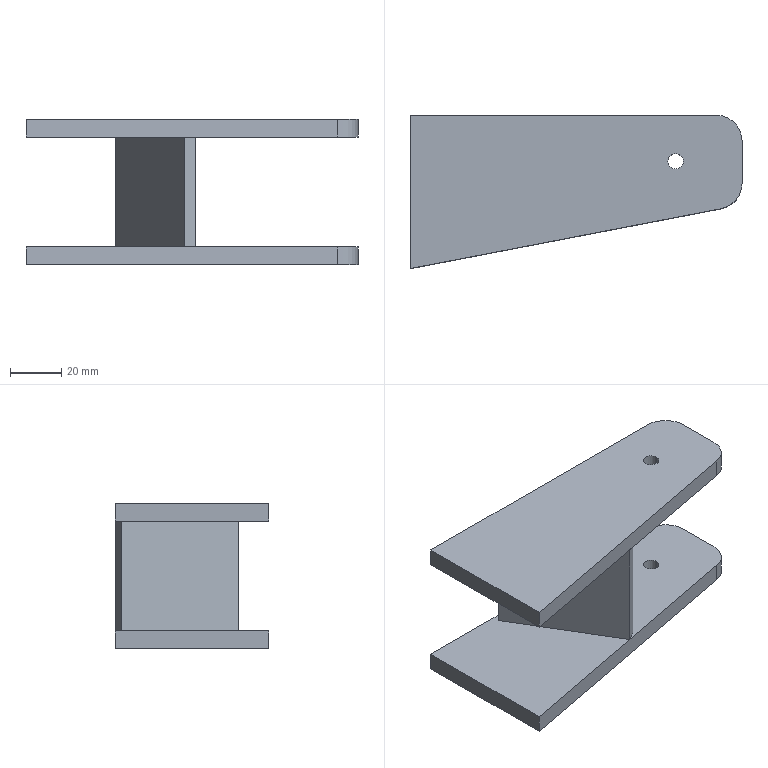Part | SolidWorks | features Cut 1, Extrusion 1, Fillet 1, ICE 1, LPattern 1 | 3 solids | 26 faces | box 130 x 60 x 57 mm | volume 96959 mm3 | plane 18 | cylinder 8 | commonest cylinder face diameters 6 x4 20 x4
STEP:
#1=CARTESIAN_POINT('',(793.,104.,-1688.));
#2=VERTEX_POINT('',#1);
#3=CARTESIAN_POINT('',(787.,104.,-1688.));
#4=VERTEX_POINT('',#3);
#5=CARTESIAN_POINT('',(790.,104.,-1688.));
#6=DIRECTION('',(0.,0.,-1.));
#7=DIRECTION('',(-1.,0.,0.));
#8=AXIS2_PLACEMENT_3D('',#5,#6,#7);
#9=CIRCLE('',#8,3.);
#10=EDGE_CURVE('',#2,#4,#9,.T.);
#11=ORIENTED_EDGE('',*,*,#10,.F.);
#12=CARTESIAN_POINT('',(793.,104.,-1695.));
#13=VERTEX_POINT('',#12);
#14=CARTESIAN_POINT('',(793.,104.,-1688.));
#15=DIRECTION('',(0.,0.,-1.));
#16=VECTOR('',#15,1000.);
#17=LINE('',#14,#16);
#18=EDGE_CURVE('',#2,#13,#17,.T.);
#19=ORIENTED_EDGE('',*,*,#18,.T.);
#20=CARTESIAN_POINT('',(787.,104.,-1695.));
#21=VERTEX_POINT('',#20);
#22=CARTESIAN_POINT('',(790.,104.,-1695.));
#23=DIRECTION('',(0.,0.,-1.));
#24=DIRECTION('',(-1.,0.,0.));
#25=AXIS2_PLACEMENT_3D('',#22,#23,#24);
#26=CIRCLE('',#25,3.);
#27=EDGE_CURVE('',#13,#21,#26,.T.);
#28=ORIENTED_EDGE('',*,*,#27,.T.);
#29=CARTESIAN_POINT('',(787.,104.,-1688.));
#30=DIRECTION('',(0.,0.,-1.));
#31=VECTOR('',#30,1000.);
#32=LINE('',#29,#31);
#33=EDGE_CURVE('',#4,#21,#32,.T.);
#34=ORIENTED_EDGE('',*,*,#33,.F.);
#35=EDGE_LOOP('',(#11,#19,#28,#34));
#36=FACE_OUTER_BOUND('',#35,.T.);
#37=CARTESIAN_POINT('',(790.,104.,-1688.));
#38=DIRECTION('',(0.,0.,-1.));
#39=DIRECTION('',(-1.,0.,0.));
#40=AXIS2_PLACEMENT_3D('',#37,#38,#39);
#41=CYLINDRICAL_SURFACE('',#40,3.);
#42=ADVANCED_FACE('',(#36),#41,.F.);
#43=CARTESIAN_POINT('',(790.,104.,-1688.));
#44=DIRECTION('',(0.,0.,-1.));
#45=DIRECTION('',(-1.,0.,0.));
#46=AXIS2_PLACEMENT_3D('',#43,#44,#45);
#47=CIRCLE('',#46,3.);
#48=EDGE_CURVE('',#4,#2,#47,.T.);
#49=ORIENTED_EDGE('',*,*,#48,.T.);
#50=ORIENTED_EDGE('',*,*,#10,.T.);
#51=EDGE_LOOP('',(#49,#50));
#52=FACE_BOUND('',#51,.T.);
#53=CARTESIAN_POINT('',(816.,112.,-1688.));
#54=VERTEX_POINT('',#53);
#55=CARTESIAN_POINT('',(816.,95.26,-1688.));
#56=VERTEX_POINT('',#55);
#57=CARTESIAN_POINT('',(816.,122.,-1688.));
#58=DIRECTION('',(0.,-1.,0.));
#59=VECTOR('',#58,1000.);
#60=LINE('',#57,#59);
#61=EDGE_CURVE('',#54,#56,#60,.T.);
#62=ORIENTED_EDGE('',*,*,#61,.F.);
#63=CARTESIAN_POINT('',(806.,122.,-1688.));
#64=VERTEX_POINT('',#63);
#65=CARTESIAN_POINT('',(806.,112.,-1688.));
#66=DIRECTION('',(0.,0.,1.));
#67=DIRECTION('',(-1.,0.,0.));
#68=AXIS2_PLACEMENT_3D('',#65,#66,#67);
#69=CIRCLE('',#68,10.);
#70=EDGE_CURVE('',#54,#64,#69,.T.);
#71=ORIENTED_EDGE('',*,*,#70,.T.);
#72=CARTESIAN_POINT('',(686.,122.,-1688.));
#73=VERTEX_POINT('',#72);
#74=CARTESIAN_POINT('',(816.,122.,-1688.));
#75=DIRECTION('',(-1.,0.,0.));
#76=VECTOR('',#75,1000.);
#77=LINE('',#74,#76);
#78=EDGE_CURVE('',#64,#73,#77,.T.);
#79=ORIENTED_EDGE('',*,*,#78,.T.);
#80=CARTESIAN_POINT('',(686.,62.,-1688.));
#81=VERTEX_POINT('',#80);
#82=CARTESIAN_POINT('',(686.,122.,-1688.));
#83=DIRECTION('',(0.,-1.,0.));
#84=VECTOR('',#83,1000.);
#85=LINE('',#82,#84);
#86=EDGE_CURVE('',#73,#81,#85,.T.);
#87=ORIENTED_EDGE('',*,*,#86,.T.);
#88=CARTESIAN_POINT('',(807.888,85.44,-1688.));
#89=VERTEX_POINT('',#88);
#90=CARTESIAN_POINT('',(816.,87.,-1688.));
#91=DIRECTION('',(0.982,0.1888,0.));
#92=VECTOR('',#91,1000.);
#93=LINE('',#90,#92);
#94=EDGE_CURVE('',#81,#89,#93,.T.);
#95=ORIENTED_EDGE('',*,*,#94,.T.);
#96=CARTESIAN_POINT('',(806.,95.26,-1688.));
#97=DIRECTION('',(0.,0.,1.));
#98=DIRECTION('',(-1.,0.,0.));
#99=AXIS2_PLACEMENT_3D('',#96,#97,#98);
#100=CIRCLE('',#99,10.);
#101=EDGE_CURVE('',#89,#56,#100,.T.);
#102=ORIENTED_EDGE('',*,*,#101,.T.);
#103=EDGE_LOOP('',(#62,#71,#79,#87,#95,#102));
#104=FACE_OUTER_BOUND('',#103,.T.);
#105=CARTESIAN_POINT('',(816.,122.,-1688.));
#106=DIRECTION('',(0.,0.,-1.));
#107=DIRECTION('',(-1.,0.,0.));
#108=AXIS2_PLACEMENT_3D('',#105,#106,#107);
#109=PLANE('',#108);
#110=ADVANCED_FACE('',(#52,#104),#109,.F.);
#111=CARTESIAN_POINT('',(790.,104.,-1695.));
#112=DIRECTION('',(0.,0.,-1.));
#113=DIRECTION('',(-1.,0.,0.));
#114=AXIS2_PLACEMENT_3D('',#111,#112,#113);
#115=CIRCLE('',#114,3.);
#116=EDGE_CURVE('',#21,#13,#115,.T.);
#117=ORIENTED_EDGE('',*,*,#116,.F.);
#118=ORIENTED_EDGE('',*,*,#27,.F.);
#119=EDGE_LOOP('',(#117,#118));
#120=FACE_BOUND('',#119,.T.);
#121=CARTESIAN_POINT('',(806.,122.,-1695.));
#122=VERTEX_POINT('',#121);
#123=CARTESIAN_POINT('',(686.,122.,-1695.));
#124=VERTEX_POINT('',#123);
#125=CARTESIAN_POINT('',(816.,122.,-1695.));
#126=DIRECTION('',(-1.,0.,0.));
#127=VECTOR('',#126,1000.);
#128=LINE('',#125,#127);
#129=EDGE_CURVE('',#122,#124,#128,.T.);
#130=ORIENTED_EDGE('',*,*,#129,.F.);
#131=CARTESIAN_POINT('',(816.,112.,-1695.));
#132=VERTEX_POINT('',#131);
#133=CARTESIAN_POINT('',(806.,112.,-1695.));
#134=DIRECTION('',(0.,0.,-1.));
#135=DIRECTION('',(1.,0.,0.));
#136=AXIS2_PLACEMENT_3D('',#133,#134,#135);
#137=CIRCLE('',#136,10.);
#138=EDGE_CURVE('',#122,#132,#137,.T.);
#139=ORIENTED_EDGE('',*,*,#138,.T.);
#140=CARTESIAN_POINT('',(816.,95.26,-1695.));
#141=VERTEX_POINT('',#140);
#142=CARTESIAN_POINT('',(816.,122.,-1695.));
#143=DIRECTION('',(0.,1.,0.));
#144=VECTOR('',#143,1000.);
#145=LINE('',#142,#144);
#146=EDGE_CURVE('',#141,#132,#145,.T.);
#147=ORIENTED_EDGE('',*,*,#146,.F.);
#148=CARTESIAN_POINT('',(807.888,85.44,-1695.));
#149=VERTEX_POINT('',#148);
#150=CARTESIAN_POINT('',(806.,95.26,-1695.));
#151=DIRECTION('',(0.,0.,-1.));
#152=DIRECTION('',(1.,0.,0.));
#153=AXIS2_PLACEMENT_3D('',#150,#151,#152);
#154=CIRCLE('',#153,10.);
#155=EDGE_CURVE('',#141,#149,#154,.T.);
#156=ORIENTED_EDGE('',*,*,#155,.T.);
#157=CARTESIAN_POINT('',(686.,62.,-1695.));
#158=VERTEX_POINT('',#157);
#159=CARTESIAN_POINT('',(816.,87.,-1695.));
#160=DIRECTION('',(0.982,0.1888,0.));
#161=VECTOR('',#160,1000.);
#162=LINE('',#159,#161);
#163=EDGE_CURVE('',#158,#149,#162,.T.);
#164=ORIENTED_EDGE('',*,*,#163,.F.);
#165=CARTESIAN_POINT('',(686.,122.,-1695.));
#166=DIRECTION('',(0.,1.,0.));
#167=VECTOR('',#166,1000.);
#168=LINE('',#165,#167);
#169=EDGE_CURVE('',#158,#124,#168,.T.);
#170=ORIENTED_EDGE('',*,*,#169,.T.);
#171=EDGE_LOOP('',(#130,#139,#147,#156,#164,#170));
#172=FACE_OUTER_BOUND('',#171,.T.);
#173=CARTESIAN_POINT('',(816.,122.,-1695.));
#174=DIRECTION('',(0.,0.,1.));
#175=DIRECTION('',(1.,0.,0.));
#176=AXIS2_PLACEMENT_3D('',#173,#174,#175);
#177=PLANE('',#176);
#178=ADVANCED_FACE('',(#120,#172),#177,.F.);
#179=ORIENTED_EDGE('',*,*,#78,.F.);
#180=CARTESIAN_POINT('',(806.,122.,-1695.));
#181=DIRECTION('',(0.,0.,-1.));
#182=VECTOR('',#181,1000.);
#183=LINE('',#180,#182);
#184=EDGE_CURVE('',#64,#122,#183,.T.);
#185=ORIENTED_EDGE('',*,*,#184,.T.);
#186=ORIENTED_EDGE('',*,*,#129,.T.);
#187=CARTESIAN_POINT('',(686.,122.,-1688.));
#188=DIRECTION('',(0.,0.,1.));
#189=VECTOR('',#188,1000.);
#190=LINE('',#187,#189);
#191=EDGE_CURVE('',#124,#73,#190,.T.);
#192=ORIENTED_EDGE('',*,*,#191,.T.);
#193=EDGE_LOOP('',(#179,#185,#186,#192));
#194=FACE_OUTER_BOUND('',#193,.T.);
#195=CARTESIAN_POINT('',(816.,122.,-1688.));
#196=DIRECTION('',(0.,-1.,0.));
#197=DIRECTION('',(0.,0.,-1.));
#198=AXIS2_PLACEMENT_3D('',#195,#196,#197);
#199=PLANE('',#198);
#200=ADVANCED_FACE('',(#194),#199,.F.);
#201=ORIENTED_EDGE('',*,*,#146,.T.);
#202=CARTESIAN_POINT('',(816.,112.,-1688.));
#203=DIRECTION('',(0.,0.,1.));
#204=VECTOR('',#203,1000.);
#205=LINE('',#202,#204);
#206=EDGE_CURVE('',#132,#54,#205,.T.);
#207=ORIENTED_EDGE('',*,*,#206,.T.);
#208=ORIENTED_EDGE('',*,*,#61,.T.);
#209=CARTESIAN_POINT('',(816.,95.26,-1695.));
#210=DIRECTION('',(0.,0.,-1.));
#211=VECTOR('',#210,1000.);
#212=LINE('',#209,#211);
#213=EDGE_CURVE('',#56,#141,#212,.T.);
#214=ORIENTED_EDGE('',*,*,#213,.T.);
#215=EDGE_LOOP('',(#201,#207,#208,#214));
#216=FACE_OUTER_BOUND('',#215,.T.);
#217=CARTESIAN_POINT('',(816.,62.,-1688.));
#218=DIRECTION('',(1.,0.,0.));
#219=DIRECTION('',(0.,0.,-1.));
#220=AXIS2_PLACEMENT_3D('',#217,#218,#219);
#221=PLANE('',#220);
#222=ADVANCED_FACE('',(#216),#221,.T.);
#223=ORIENTED_EDGE('',*,*,#86,.F.);
#224=ORIENTED_EDGE('',*,*,#191,.F.);
#225=ORIENTED_EDGE('',*,*,#169,.F.);
#226=CARTESIAN_POINT('',(686.,62.,-1688.));
#227=DIRECTION('',(0.,0.,-1.));
#228=VECTOR('',#227,1000.);
#229=LINE('',#226,#228);
#230=EDGE_CURVE('',#81,#158,#229,.T.);
#231=ORIENTED_EDGE('',*,*,#230,.F.);
#232=EDGE_LOOP('',(#223,#224,#225,#231));
#233=FACE_OUTER_BOUND('',#232,.T.);
#234=CARTESIAN_POINT('',(686.,62.,-1688.));
#235=DIRECTION('',(1.,0.,0.));
#236=DIRECTION('',(0.,0.,-1.));
#237=AXIS2_PLACEMENT_3D('',#234,#235,#236);
#238=PLANE('',#237);
#239=ADVANCED_FACE('',(#233),#238,.F.);
#240=ORIENTED_EDGE('',*,*,#163,.T.);
#241=CARTESIAN_POINT('',(807.888,85.44,-1688.));
#242=DIRECTION('',(0.,0.,1.));
#243=VECTOR('',#242,1000.);
#244=LINE('',#241,#243);
#245=EDGE_CURVE('',#149,#89,#244,.T.);
#246=ORIENTED_EDGE('',*,*,#245,.T.);
#247=ORIENTED_EDGE('',*,*,#94,.F.);
#248=ORIENTED_EDGE('',*,*,#230,.T.);
#249=EDGE_LOOP('',(#240,#246,#247,#248));
#250=FACE_OUTER_BOUND('',#249,.T.);
#251=CARTESIAN_POINT('',(816.,87.,-1688.));
#252=DIRECTION('',(-0.1888,0.982,0.));
#253=DIRECTION('',(-0.982,-0.1888,0.));
#254=AXIS2_PLACEMENT_3D('',#251,#252,#253);
#255=PLANE('',#254);
#256=ADVANCED_FACE('',(#250),#255,.F.);
#257=ORIENTED_EDGE('',*,*,#18,.F.);
#258=ORIENTED_EDGE('',*,*,#48,.F.);
#259=ORIENTED_EDGE('',*,*,#33,.T.);
#260=ORIENTED_EDGE('',*,*,#116,.T.);
#261=EDGE_LOOP('',(#257,#258,#259,#260));
#262=FACE_OUTER_BOUND('',#261,.T.);
#263=CARTESIAN_POINT('',(790.,104.,-1688.));
#264=DIRECTION('',(0.,0.,-1.));
#265=DIRECTION('',(-1.,0.,0.));
#266=AXIS2_PLACEMENT_3D('',#263,#264,#265);
#267=CYLINDRICAL_SURFACE('',#266,3.);
#268=ADVANCED_FACE('',(#262),#267,.F.);
#269=ORIENTED_EDGE('',*,*,#138,.F.);
#270=ORIENTED_EDGE('',*,*,#184,.F.);
#271=ORIENTED_EDGE('',*,*,#70,.F.);
#272=ORIENTED_EDGE('',*,*,#206,.F.);
#273=EDGE_LOOP('',(#269,#270,#271,#272));
#274=FACE_OUTER_BOUND('',#273,.T.);
#275=CARTESIAN_POINT('',(806.,112.,-1688.));
#276=DIRECTION('',(0.,0.,-1.));
#277=DIRECTION('',(-1.,0.,0.));
#278=AXIS2_PLACEMENT_3D('',#275,#276,#277);
#279=CYLINDRICAL_SURFACE('',#278,10.);
#280=ADVANCED_FACE('',(#274),#279,.T.);
#281=ORIENTED_EDGE('',*,*,#101,.F.);
#282=ORIENTED_EDGE('',*,*,#245,.F.);
#283=ORIENTED_EDGE('',*,*,#155,.F.);
#284=ORIENTED_EDGE('',*,*,#213,.F.);
#285=EDGE_LOOP('',(#281,#282,#283,#284));
#286=FACE_OUTER_BOUND('',#285,.T.);
#287=CARTESIAN_POINT('',(806.,95.26,-1688.));
#288=DIRECTION('',(0.,0.,1.));
#289=DIRECTION('',(1.,0.,0.));
#290=AXIS2_PLACEMENT_3D('',#287,#288,#289);
#291=CYLINDRICAL_SURFACE('',#290,10.);
#292=ADVANCED_FACE('',(#286),#291,.T.);
#293=CLOSED_SHELL('',(#42,#110,#178,#200,#222,#239,#256,#268,#280,#292));
#294=MANIFOLD_SOLID_BREP('',#293);
#295=CARTESIAN_POINT('',(793.,104.,-1638.));
#296=VERTEX_POINT('',#295);
#297=CARTESIAN_POINT('',(787.,104.,-1638.));
#298=VERTEX_POINT('',#297);
#299=CARTESIAN_POINT('',(790.,104.,-1638.));
#300=DIRECTION('',(0.,0.,-1.));
#301=DIRECTION('',(-1.,0.,0.));
#302=AXIS2_PLACEMENT_3D('',#299,#300,#301);
#303=CIRCLE('',#302,3.);
#304=EDGE_CURVE('',#296,#298,#303,.T.);
#305=ORIENTED_EDGE('',*,*,#304,.F.);
#306=CARTESIAN_POINT('',(793.,104.,-1645.));
#307=VERTEX_POINT('',#306);
#308=CARTESIAN_POINT('',(793.,104.,-1638.));
#309=DIRECTION('',(0.,0.,-1.));
#310=VECTOR('',#309,1000.);
#311=LINE('',#308,#310);
#312=EDGE_CURVE('',#296,#307,#311,.T.);
#313=ORIENTED_EDGE('',*,*,#312,.T.);
#314=CARTESIAN_POINT('',(787.,104.,-1645.));
#315=VERTEX_POINT('',#314);
#316=CARTESIAN_POINT('',(790.,104.,-1645.));
#317=DIRECTION('',(0.,0.,-1.));
#318=DIRECTION('',(-1.,0.,0.));
#319=AXIS2_PLACEMENT_3D('',#316,#317,#318);
#320=CIRCLE('',#319,3.);
#321=EDGE_CURVE('',#307,#315,#320,.T.);
#322=ORIENTED_EDGE('',*,*,#321,.T.);
#323=CARTESIAN_POINT('',(787.,104.,-1638.));
#324=DIRECTION('',(0.,0.,-1.));
#325=VECTOR('',#324,1000.);
#326=LINE('',#323,#325);
#327=EDGE_CURVE('',#298,#315,#326,.T.);
#328=ORIENTED_EDGE('',*,*,#327,.F.);
#329=EDGE_LOOP('',(#305,#313,#322,#328));
#330=FACE_OUTER_BOUND('',#329,.T.);
#331=CARTESIAN_POINT('',(790.,104.,-1638.));
#332=DIRECTION('',(0.,0.,-1.));
#333=DIRECTION('',(-1.,0.,0.));
#334=AXIS2_PLACEMENT_3D('',#331,#332,#333);
#335=CYLINDRICAL_SURFACE('',#334,3.);
#336=ADVANCED_FACE('',(#330),#335,.F.);
#337=CARTESIAN_POINT('',(790.,104.,-1638.));
#338=DIRECTION('',(0.,0.,-1.));
#339=DIRECTION('',(-1.,0.,0.));
#340=AXIS2_PLACEMENT_3D('',#337,#338,#339);
#341=CIRCLE('',#340,3.);
#342=EDGE_CURVE('',#298,#296,#341,.T.);
#343=ORIENTED_EDGE('',*,*,#342,.T.);
#344=ORIENTED_EDGE('',*,*,#304,.T.);
#345=EDGE_LOOP('',(#343,#344));
#346=FACE_BOUND('',#345,.T.);
#347=CARTESIAN_POINT('',(816.,112.,-1638.));
#348=VERTEX_POINT('',#347);
#349=CARTESIAN_POINT('',(816.,95.26,-1638.));
#350=VERTEX_POINT('',#349);
#351=CARTESIAN_POINT('',(816.,122.,-1638.));
#352=DIRECTION('',(0.,-1.,0.));
#353=VECTOR('',#352,1000.);
#354=LINE('',#351,#353);
#355=EDGE_CURVE('',#348,#350,#354,.T.);
#356=ORIENTED_EDGE('',*,*,#355,.F.);
#357=CARTESIAN_POINT('',(806.,122.,-1638.));
#358=VERTEX_POINT('',#357);
#359=CARTESIAN_POINT('',(806.,112.,-1638.));
#360=DIRECTION('',(0.,0.,1.));
#361=DIRECTION('',(-1.,0.,0.));
#362=AXIS2_PLACEMENT_3D('',#359,#360,#361);
#363=CIRCLE('',#362,10.);
#364=EDGE_CURVE('',#348,#358,#363,.T.);
#365=ORIENTED_EDGE('',*,*,#364,.T.);
#366=CARTESIAN_POINT('',(686.,122.,-1638.));
#367=VERTEX_POINT('',#366);
#368=CARTESIAN_POINT('',(816.,122.,-1638.));
#369=DIRECTION('',(-1.,0.,0.));
#370=VECTOR('',#369,1000.);
#371=LINE('',#368,#370);
#372=EDGE_CURVE('',#358,#367,#371,.T.);
#373=ORIENTED_EDGE('',*,*,#372,.T.);
#374=CARTESIAN_POINT('',(686.,62.,-1638.));
#375=VERTEX_POINT('',#374);
#376=CARTESIAN_POINT('',(686.,122.,-1638.));
#377=DIRECTION('',(0.,-1.,0.));
#378=VECTOR('',#377,1000.);
#379=LINE('',#376,#378);
#380=EDGE_CURVE('',#367,#375,#379,.T.);
#381=ORIENTED_EDGE('',*,*,#380,.T.);
#382=CARTESIAN_POINT('',(807.888,85.44,-1638.));
#383=VERTEX_POINT('',#382);
#384=CARTESIAN_POINT('',(816.,87.,-1638.));
#385=DIRECTION('',(0.982,0.1888,0.));
#386=VECTOR('',#385,1000.);
#387=LINE('',#384,#386);
#388=EDGE_CURVE('',#375,#383,#387,.T.);
#389=ORIENTED_EDGE('',*,*,#388,.T.);
#390=CARTESIAN_POINT('',(806.,95.26,-1638.));
#391=DIRECTION('',(0.,0.,1.));
#392=DIRECTION('',(-1.,0.,0.));
#393=AXIS2_PLACEMENT_3D('',#390,#391,#392);
#394=CIRCLE('',#393,10.);
#395=EDGE_CURVE('',#383,#350,#394,.T.);
#396=ORIENTED_EDGE('',*,*,#395,.T.);
#397=EDGE_LOOP('',(#356,#365,#373,#381,#389,#396));
#398=FACE_OUTER_BOUND('',#397,.T.);
#399=CARTESIAN_POINT('',(816.,122.,-1638.));
#400=DIRECTION('',(0.,0.,-1.));
#401=DIRECTION('',(-1.,0.,0.));
#402=AXIS2_PLACEMENT_3D('',#399,#400,#401);
#403=PLANE('',#402);
#404=ADVANCED_FACE('',(#346,#398),#403,.F.);
#405=CARTESIAN_POINT('',(790.,104.,-1645.));
#406=DIRECTION('',(0.,0.,-1.));
#407=DIRECTION('',(-1.,0.,0.));
#408=AXIS2_PLACEMENT_3D('',#405,#406,#407);
#409=CIRCLE('',#408,3.);
#410=EDGE_CURVE('',#315,#307,#409,.T.);
#411=ORIENTED_EDGE('',*,*,#410,.F.);
#412=ORIENTED_EDGE('',*,*,#321,.F.);
#413=EDGE_LOOP('',(#411,#412));
#414=FACE_BOUND('',#413,.T.);
#415=CARTESIAN_POINT('',(806.,122.,-1645.));
#416=VERTEX_POINT('',#415);
#417=CARTESIAN_POINT('',(686.,122.,-1645.));
#418=VERTEX_POINT('',#417);
#419=CARTESIAN_POINT('',(816.,122.,-1645.));
#420=DIRECTION('',(-1.,0.,0.));
#421=VECTOR('',#420,1000.);
#422=LINE('',#419,#421);
#423=EDGE_CURVE('',#416,#418,#422,.T.);
#424=ORIENTED_EDGE('',*,*,#423,.F.);
#425=CARTESIAN_POINT('',(816.,112.,-1645.));
#426=VERTEX_POINT('',#425);
#427=CARTESIAN_POINT('',(806.,112.,-1645.));
#428=DIRECTION('',(0.,0.,-1.));
#429=DIRECTION('',(1.,0.,0.));
#430=AXIS2_PLACEMENT_3D('',#427,#428,#429);
#431=CIRCLE('',#430,10.);
#432=EDGE_CURVE('',#416,#426,#431,.T.);
#433=ORIENTED_EDGE('',*,*,#432,.T.);
#434=CARTESIAN_POINT('',(816.,95.26,-1645.));
#435=VERTEX_POINT('',#434);
#436=CARTESIAN_POINT('',(816.,122.,-1645.));
#437=DIRECTION('',(0.,1.,0.));
#438=VECTOR('',#437,1000.);
#439=LINE('',#436,#438);
#440=EDGE_CURVE('',#435,#426,#439,.T.);
#441=ORIENTED_EDGE('',*,*,#440,.F.);
#442=CARTESIAN_POINT('',(807.888,85.44,-1645.));
#443=VERTEX_POINT('',#442);
#444=CARTESIAN_POINT('',(806.,95.26,-1645.));
#445=DIRECTION('',(0.,0.,-1.));
#446=DIRECTION('',(1.,0.,0.));
#447=AXIS2_PLACEMENT_3D('',#444,#445,#446);
#448=CIRCLE('',#447,10.);
#449=EDGE_CURVE('',#435,#443,#448,.T.);
#450=ORIENTED_EDGE('',*,*,#449,.T.);
#451=CARTESIAN_POINT('',(686.,62.,-1645.));
#452=VERTEX_POINT('',#451);
#453=CARTESIAN_POINT('',(816.,87.,-1645.));
#454=DIRECTION('',(0.982,0.1888,0.));
#455=VECTOR('',#454,1000.);
#456=LINE('',#453,#455);
#457=EDGE_CURVE('',#452,#443,#456,.T.);
#458=ORIENTED_EDGE('',*,*,#457,.F.);
#459=CARTESIAN_POINT('',(686.,122.,-1645.));
#460=DIRECTION('',(0.,1.,0.));
#461=VECTOR('',#460,1000.);
#462=LINE('',#459,#461);
#463=EDGE_CURVE('',#452,#418,#462,.T.);
#464=ORIENTED_EDGE('',*,*,#463,.T.);
#465=EDGE_LOOP('',(#424,#433,#441,#450,#458,#464));
#466=FACE_OUTER_BOUND('',#465,.T.);
#467=CARTESIAN_POINT('',(816.,122.,-1645.));
#468=DIRECTION('',(0.,0.,1.));
#469=DIRECTION('',(1.,0.,0.));
#470=AXIS2_PLACEMENT_3D('',#467,#468,#469);
#471=PLANE('',#470);
#472=ADVANCED_FACE('',(#414,#466),#471,.F.);
#473=ORIENTED_EDGE('',*,*,#372,.F.);
#474=CARTESIAN_POINT('',(806.,122.,-1645.));
#475=DIRECTION('',(0.,0.,-1.));
#476=VECTOR('',#475,1000.);
#477=LINE('',#474,#476);
#478=EDGE_CURVE('',#358,#416,#477,.T.);
#479=ORIENTED_EDGE('',*,*,#478,.T.);
#480=ORIENTED_EDGE('',*,*,#423,.T.);
#481=CARTESIAN_POINT('',(686.,122.,-1638.));
#482=DIRECTION('',(0.,0.,1.));
#483=VECTOR('',#482,1000.);
#484=LINE('',#481,#483);
#485=EDGE_CURVE('',#418,#367,#484,.T.);
#486=ORIENTED_EDGE('',*,*,#485,.T.);
#487=EDGE_LOOP('',(#473,#479,#480,#486));
#488=FACE_OUTER_BOUND('',#487,.T.);
#489=CARTESIAN_POINT('',(816.,122.,-1638.));
#490=DIRECTION('',(0.,-1.,0.));
#491=DIRECTION('',(0.,0.,-1.));
#492=AXIS2_PLACEMENT_3D('',#489,#490,#491);
#493=PLANE('',#492);
#494=ADVANCED_FACE('',(#488),#493,.F.);
#495=ORIENTED_EDGE('',*,*,#440,.T.);
#496=CARTESIAN_POINT('',(816.,112.,-1638.));
#497=DIRECTION('',(0.,0.,1.));
#498=VECTOR('',#497,1000.);
#499=LINE('',#496,#498);
#500=EDGE_CURVE('',#426,#348,#499,.T.);
#501=ORIENTED_EDGE('',*,*,#500,.T.);
#502=ORIENTED_EDGE('',*,*,#355,.T.);
#503=CARTESIAN_POINT('',(816.,95.26,-1645.));
#504=DIRECTION('',(0.,0.,-1.));
#505=VECTOR('',#504,1000.);
#506=LINE('',#503,#505);
#507=EDGE_CURVE('',#350,#435,#506,.T.);
#508=ORIENTED_EDGE('',*,*,#507,.T.);
#509=EDGE_LOOP('',(#495,#501,#502,#508));
#510=FACE_OUTER_BOUND('',#509,.T.);
#511=CARTESIAN_POINT('',(816.,62.,-1638.));
#512=DIRECTION('',(1.,0.,0.));
#513=DIRECTION('',(0.,0.,-1.));
#514=AXIS2_PLACEMENT_3D('',#511,#512,#513);
#515=PLANE('',#514);
#516=ADVANCED_FACE('',(#510),#515,.T.);
#517=ORIENTED_EDGE('',*,*,#380,.F.);
#518=ORIENTED_EDGE('',*,*,#485,.F.);
#519=ORIENTED_EDGE('',*,*,#463,.F.);
#520=CARTESIAN_POINT('',(686.,62.,-1638.));
#521=DIRECTION('',(0.,0.,-1.));
#522=VECTOR('',#521,1000.);
#523=LINE('',#520,#522);
#524=EDGE_CURVE('',#375,#452,#523,.T.);
#525=ORIENTED_EDGE('',*,*,#524,.F.);
#526=EDGE_LOOP('',(#517,#518,#519,#525));
#527=FACE_OUTER_BOUND('',#526,.T.);
#528=CARTESIAN_POINT('',(686.,62.,-1638.));
#529=DIRECTION('',(1.,0.,0.));
#530=DIRECTION('',(0.,0.,-1.));
#531=AXIS2_PLACEMENT_3D('',#528,#529,#530);
#532=PLANE('',#531);
#533=ADVANCED_FACE('',(#527),#532,.F.);
#534=ORIENTED_EDGE('',*,*,#457,.T.);
#535=CARTESIAN_POINT('',(807.888,85.44,-1638.));
#536=DIRECTION('',(0.,0.,1.));
#537=VECTOR('',#536,1000.);
#538=LINE('',#535,#537);
#539=EDGE_CURVE('',#443,#383,#538,.T.);
#540=ORIENTED_EDGE('',*,*,#539,.T.);
#541=ORIENTED_EDGE('',*,*,#388,.F.);
#542=ORIENTED_EDGE('',*,*,#524,.T.);
#543=EDGE_LOOP('',(#534,#540,#541,#542));
#544=FACE_OUTER_BOUND('',#543,.T.);
#545=CARTESIAN_POINT('',(816.,87.,-1638.));
#546=DIRECTION('',(-0.1888,0.982,0.));
#547=DIRECTION('',(-0.982,-0.1888,0.));
#548=AXIS2_PLACEMENT_3D('',#545,#546,#547);
#549=PLANE('',#548);
#550=ADVANCED_FACE('',(#544),#549,.F.);
#551=ORIENTED_EDGE('',*,*,#312,.F.);
#552=ORIENTED_EDGE('',*,*,#342,.F.);
#553=ORIENTED_EDGE('',*,*,#327,.T.);
#554=ORIENTED_EDGE('',*,*,#410,.T.);
#555=EDGE_LOOP('',(#551,#552,#553,#554));
#556=FACE_OUTER_BOUND('',#555,.T.);
#557=CARTESIAN_POINT('',(790.,104.,-1638.));
#558=DIRECTION('',(0.,0.,-1.));
#559=DIRECTION('',(-1.,0.,0.));
#560=AXIS2_PLACEMENT_3D('',#557,#558,#559);
#561=CYLINDRICAL_SURFACE('',#560,3.);
#562=ADVANCED_FACE('',(#556),#561,.F.);
#563=ORIENTED_EDGE('',*,*,#432,.F.);
#564=ORIENTED_EDGE('',*,*,#478,.F.);
#565=ORIENTED_EDGE('',*,*,#364,.F.);
#566=ORIENTED_EDGE('',*,*,#500,.F.);
#567=EDGE_LOOP('',(#563,#564,#565,#566));
#568=FACE_OUTER_BOUND('',#567,.T.);
#569=CARTESIAN_POINT('',(806.,112.,-1638.));
#570=DIRECTION('',(0.,0.,-1.));
#571=DIRECTION('',(-1.,0.,0.));
#572=AXIS2_PLACEMENT_3D('',#569,#570,#571);
#573=CYLINDRICAL_SURFACE('',#572,10.);
#574=ADVANCED_FACE('',(#568),#573,.T.);
#575=ORIENTED_EDGE('',*,*,#395,.F.);
#576=ORIENTED_EDGE('',*,*,#539,.F.);
#577=ORIENTED_EDGE('',*,*,#449,.F.);
#578=ORIENTED_EDGE('',*,*,#507,.F.);
#579=EDGE_LOOP('',(#575,#576,#577,#578));
#580=FACE_OUTER_BOUND('',#579,.T.);
#581=CARTESIAN_POINT('',(806.,95.26,-1638.));
#582=DIRECTION('',(0.,0.,1.));
#583=DIRECTION('',(1.,0.,0.));
#584=AXIS2_PLACEMENT_3D('',#581,#582,#583);
#585=CYLINDRICAL_SURFACE('',#584,10.);
#586=ADVANCED_FACE('',(#580),#585,.T.);
#587=CLOSED_SHELL('',(#336,#404,#472,#494,#516,#533,#550,#562,#574,#586));
#588=MANIFOLD_SOLID_BREP('',#587);
#589=CARTESIAN_POINT('',(748.135,73.949,-1645.));
#590=VERTEX_POINT('',#589);
#591=CARTESIAN_POINT('',(752.426,76.516,-1645.));
#592=VERTEX_POINT('',#591);
#593=CARTESIAN_POINT('',(748.135,73.949,-1645.));
#594=DIRECTION('',(0.8582,0.5133,0.));
#595=VECTOR('',#594,1000.);
#596=LINE('',#593,#595);
#597=EDGE_CURVE('',#590,#592,#596,.T.);
#598=ORIENTED_EDGE('',*,*,#597,.T.);
#599=CARTESIAN_POINT('',(725.22,122.,-1645.));
#600=VERTEX_POINT('',#599);
#601=CARTESIAN_POINT('',(752.426,76.516,-1645.));
#602=DIRECTION('',(-0.5133,0.8582,0.));
#603=VECTOR('',#602,1000.);
#604=LINE('',#601,#603);
#605=EDGE_CURVE('',#592,#600,#604,.T.);
#606=ORIENTED_EDGE('',*,*,#605,.T.);
#607=CARTESIAN_POINT('',(720.929,119.433,-1645.));
#608=VERTEX_POINT('',#607);
#609=CARTESIAN_POINT('',(725.22,122.,-1645.));
#610=DIRECTION('',(-0.8582,-0.5133,0.));
#611=VECTOR('',#610,1000.);
#612=LINE('',#609,#611);
#613=EDGE_CURVE('',#600,#608,#612,.T.);
#614=ORIENTED_EDGE('',*,*,#613,.T.);
#615=CARTESIAN_POINT('',(720.929,119.433,-1645.));
#616=DIRECTION('',(0.5133,-0.8582,0.));
#617=VECTOR('',#616,1000.);
#618=LINE('',#615,#617);
#619=EDGE_CURVE('',#608,#590,#618,.T.);
#620=ORIENTED_EDGE('',*,*,#619,.T.);
#621=EDGE_LOOP('',(#598,#606,#614,#620));
#622=FACE_OUTER_BOUND('',#621,.T.);
#623=CARTESIAN_POINT('',(816.,122.,-1645.));
#624=DIRECTION('',(0.,0.,1.));
#625=DIRECTION('',(1.,0.,0.));
#626=AXIS2_PLACEMENT_3D('',#623,#624,#625);
#627=PLANE('',#626);
#628=ADVANCED_FACE('',(#622),#627,.T.);
#629=CARTESIAN_POINT('',(748.135,73.949,-1688.));
#630=VERTEX_POINT('',#629);
#631=CARTESIAN_POINT('',(752.426,76.516,-1688.));
#632=VERTEX_POINT('',#631);
#633=CARTESIAN_POINT('',(748.135,73.949,-1688.));
#634=DIRECTION('',(0.8582,0.5133,0.));
#635=VECTOR('',#634,1000.);
#636=LINE('',#633,#635);
#637=EDGE_CURVE('',#630,#632,#636,.T.);
#638=ORIENTED_EDGE('',*,*,#637,.F.);
#639=CARTESIAN_POINT('',(720.929,119.433,-1688.));
#640=VERTEX_POINT('',#639);
#641=CARTESIAN_POINT('',(720.929,119.433,-1688.));
#642=DIRECTION('',(0.5133,-0.8582,0.));
#643=VECTOR('',#642,1000.);
#644=LINE('',#641,#643);
#645=EDGE_CURVE('',#640,#630,#644,.T.);
#646=ORIENTED_EDGE('',*,*,#645,.F.);
#647=CARTESIAN_POINT('',(725.22,122.,-1688.));
#648=VERTEX_POINT('',#647);
#649=CARTESIAN_POINT('',(725.22,122.,-1688.));
#650=DIRECTION('',(-0.8582,-0.5133,0.));
#651=VECTOR('',#650,1000.);
#652=LINE('',#649,#651);
#653=EDGE_CURVE('',#648,#640,#652,.T.);
#654=ORIENTED_EDGE('',*,*,#653,.F.);
#655=CARTESIAN_POINT('',(752.426,76.516,-1688.));
#656=DIRECTION('',(-0.5133,0.8582,0.));
#657=VECTOR('',#656,1000.);
#658=LINE('',#655,#657);
#659=EDGE_CURVE('',#632,#648,#658,.T.);
#660=ORIENTED_EDGE('',*,*,#659,.F.);
#661=EDGE_LOOP('',(#638,#646,#654,#660));
#662=FACE_OUTER_BOUND('',#661,.T.);
#663=CARTESIAN_POINT('',(752.426,76.516,-1688.));
#664=DIRECTION('',(0.,0.,1.));
#665=DIRECTION('',(1.,0.,0.));
#666=AXIS2_PLACEMENT_3D('',#663,#664,#665);
#667=PLANE('',#666);
#668=ADVANCED_FACE('',(#662),#667,.F.);
#669=ORIENTED_EDGE('',*,*,#619,.F.);
#670=CARTESIAN_POINT('',(720.929,119.433,500000.));
#671=DIRECTION('',(0.,0.,-1.));
#672=VECTOR('',#671,1000.);
#673=LINE('',#670,#672);
#674=EDGE_CURVE('',#608,#640,#673,.T.);
#675=ORIENTED_EDGE('',*,*,#674,.T.);
#676=ORIENTED_EDGE('',*,*,#645,.T.);
#677=CARTESIAN_POINT('',(748.135,73.949,500000.));
#678=DIRECTION('',(0.,0.,-1.));
#679=VECTOR('',#678,1000.);
#680=LINE('',#677,#679);
#681=EDGE_CURVE('',#590,#630,#680,.T.);
#682=ORIENTED_EDGE('',*,*,#681,.F.);
#683=EDGE_LOOP('',(#669,#675,#676,#682));
#684=FACE_OUTER_BOUND('',#683,.T.);
#685=CARTESIAN_POINT('',(720.929,119.433,500000.));
#686=DIRECTION('',(0.8582,0.5133,0.));
#687=DIRECTION('',(-0.5133,0.8582,0.));
#688=AXIS2_PLACEMENT_3D('',#685,#686,#687);
#689=PLANE('',#688);
#690=ADVANCED_FACE('',(#684),#689,.F.);
#691=ORIENTED_EDGE('',*,*,#613,.F.);
#692=CARTESIAN_POINT('',(725.22,122.,500000.));
#693=DIRECTION('',(0.,0.,-1.));
#694=VECTOR('',#693,1000.);
#695=LINE('',#692,#694);
#696=EDGE_CURVE('',#600,#648,#695,.T.);
#697=ORIENTED_EDGE('',*,*,#696,.T.);
#698=ORIENTED_EDGE('',*,*,#653,.T.);
#699=ORIENTED_EDGE('',*,*,#674,.F.);
#700=EDGE_LOOP('',(#691,#697,#698,#699));
#701=FACE_OUTER_BOUND('',#700,.T.);
#702=CARTESIAN_POINT('',(725.22,122.,500000.));
#703=DIRECTION('',(0.5133,-0.8582,0.));
#704=DIRECTION('',(0.8582,0.5133,0.));
#705=AXIS2_PLACEMENT_3D('',#702,#703,#704);
#706=PLANE('',#705);
#707=ADVANCED_FACE('',(#701),#706,.F.);
#708=ORIENTED_EDGE('',*,*,#605,.F.);
#709=CARTESIAN_POINT('',(752.426,76.516,500000.));
#710=DIRECTION('',(0.,0.,-1.));
#711=VECTOR('',#710,1000.);
#712=LINE('',#709,#711);
#713=EDGE_CURVE('',#592,#632,#712,.T.);
#714=ORIENTED_EDGE('',*,*,#713,.T.);
#715=ORIENTED_EDGE('',*,*,#659,.T.);
#716=ORIENTED_EDGE('',*,*,#696,.F.);
#717=EDGE_LOOP('',(#708,#714,#715,#716));
#718=FACE_OUTER_BOUND('',#717,.T.);
#719=CARTESIAN_POINT('',(752.426,76.516,500000.));
#720=DIRECTION('',(-0.8582,-0.5133,0.));
#721=DIRECTION('',(0.5133,-0.8582,0.));
#722=AXIS2_PLACEMENT_3D('',#719,#720,#721);
#723=PLANE('',#722);
#724=ADVANCED_FACE('',(#718),#723,.F.);
#725=ORIENTED_EDGE('',*,*,#597,.F.);
#726=ORIENTED_EDGE('',*,*,#681,.T.);
#727=ORIENTED_EDGE('',*,*,#637,.T.);
#728=ORIENTED_EDGE('',*,*,#713,.F.);
#729=EDGE_LOOP('',(#725,#726,#727,#728));
#730=FACE_OUTER_BOUND('',#729,.T.);
#731=CARTESIAN_POINT('',(748.135,73.949,500000.));
#732=DIRECTION('',(-0.5133,0.8582,0.));
#733=DIRECTION('',(-0.8582,-0.5133,0.));
#734=AXIS2_PLACEMENT_3D('',#731,#732,#733);
#735=PLANE('',#734);
#736=ADVANCED_FACE('',(#730),#735,.F.);
#737=CLOSED_SHELL('',(#628,#668,#690,#707,#724,#736));
#738=MANIFOLD_SOLID_BREP('',#737);
#739=CARTESIAN_POINT('',(0.,0.,0.));
#740=DIRECTION('',(0.,0.,1.));
#741=DIRECTION('',(1.,0.,0.));
#742=AXIS2_PLACEMENT_3D('',#739,#740,#741);
#743=(LENGTH_UNIT()NAMED_UNIT(*)SI_UNIT(.MILLI.,.METRE.));
#744=UNCERTAINTY_MEASURE_WITH_UNIT(LENGTH_MEASURE(0.00001),#743,'','');
#745=(NAMED_UNIT(*)PLANE_ANGLE_UNIT()SI_UNIT($,.RADIAN.));
#746=(NAMED_UNIT(*)SI_UNIT($,.STERADIAN.)SOLID_ANGLE_UNIT());
#747=(GEOMETRIC_REPRESENTATION_CONTEXT(3)GLOBAL_UNCERTAINTY_ASSIGNED_CONTEXT((#744))GLOBAL_UNIT_ASSIGNED_CONTEXT((#743,#745,#746))REPRESENTATION_CONTEXT('',''));
#748=ADVANCED_BREP_SHAPE_REPRESENTATION('',(#294,#588,#738,#742),#747);